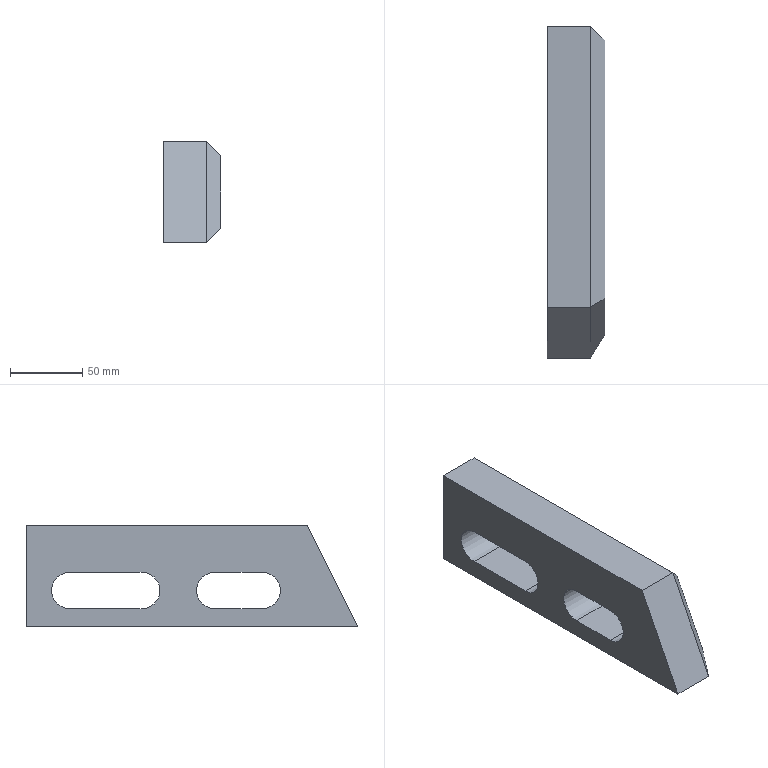Part | SolidWorks | features Chamfer 1, Extrusion 1 | 1 solid | 18 faces | box 40 x 229 x 70 mm | volume 442689 mm3 | plane 14 | cylinder 4 | commonest cylinder face diameters 25 x4
STEP:
#1=CARTESIAN_POINT('',(20.,184.,-10.));
#2=VERTEX_POINT('',#1);
#3=CARTESIAN_POINT('',(20.,6.18,-10.));
#4=VERTEX_POINT('',#3);
#5=CARTESIAN_POINT('',(20.,0.,-10.));
#6=DIRECTION('',(0.,-1.,0.));
#7=VECTOR('',#6,1000.);
#8=LINE('',#5,#7);
#9=EDGE_CURVE('',#2,#4,#8,.T.);
#10=ORIENTED_EDGE('',*,*,#9,.T.);
#11=CARTESIAN_POINT('',(20.,-18.82,-60.));
#12=VERTEX_POINT('',#11);
#13=CARTESIAN_POINT('',(20.,8.944,-4.472));
#14=DIRECTION('',(0.,-0.4472,-0.8944));
#15=VECTOR('',#14,1000.);
#16=LINE('',#13,#15);
#17=EDGE_CURVE('',#4,#12,#16,.T.);
#18=ORIENTED_EDGE('',*,*,#17,.T.);
#19=CARTESIAN_POINT('',(20.,184.,-60.));
#20=VERTEX_POINT('',#19);
#21=CARTESIAN_POINT('',(20.,0.,-60.));
#22=DIRECTION('',(0.,1.,0.));
#23=VECTOR('',#22,1000.);
#24=LINE('',#21,#23);
#25=EDGE_CURVE('',#12,#20,#24,.T.);
#26=ORIENTED_EDGE('',*,*,#25,.T.);
#27=CARTESIAN_POINT('',(20.,184.,0.));
#28=DIRECTION('',(0.,0.,1.));
#29=VECTOR('',#28,1000.);
#30=LINE('',#27,#29);
#31=EDGE_CURVE('',#20,#2,#30,.T.);
#32=ORIENTED_EDGE('',*,*,#31,.T.);
#33=EDGE_LOOP('',(#10,#18,#26,#32));
#34=FACE_OUTER_BOUND('',#33,.T.);
#35=CARTESIAN_POINT('',(20.,114.,-32.5));
#36=VERTEX_POINT('',#35);
#37=CARTESIAN_POINT('',(20.,114.,-57.5));
#38=VERTEX_POINT('',#37);
#39=CARTESIAN_POINT('',(20.,114.,-45.));
#40=DIRECTION('',(1.,0.,0.));
#41=DIRECTION('',(0.,0.,-1.));
#42=AXIS2_PLACEMENT_3D('',#39,#40,#41);
#43=CIRCLE('',#42,12.5);
#44=EDGE_CURVE('',#36,#38,#43,.T.);
#45=ORIENTED_EDGE('',*,*,#44,.F.);
#46=CARTESIAN_POINT('',(20.,164.,-32.5));
#47=VERTEX_POINT('',#46);
#48=CARTESIAN_POINT('',(20.,114.,-32.5));
#49=DIRECTION('',(0.,-1.,0.));
#50=VECTOR('',#49,1000.);
#51=LINE('',#48,#50);
#52=EDGE_CURVE('',#47,#36,#51,.T.);
#53=ORIENTED_EDGE('',*,*,#52,.F.);
#54=CARTESIAN_POINT('',(20.,164.,-57.5));
#55=VERTEX_POINT('',#54);
#56=CARTESIAN_POINT('',(20.,164.,-45.));
#57=DIRECTION('',(1.,0.,0.));
#58=DIRECTION('',(0.,0.,-1.));
#59=AXIS2_PLACEMENT_3D('',#56,#57,#58);
#60=CIRCLE('',#59,12.5);
#61=EDGE_CURVE('',#55,#47,#60,.T.);
#62=ORIENTED_EDGE('',*,*,#61,.F.);
#63=CARTESIAN_POINT('',(20.,114.,-57.5));
#64=DIRECTION('',(0.,1.,0.));
#65=VECTOR('',#64,1000.);
#66=LINE('',#63,#65);
#67=EDGE_CURVE('',#38,#55,#66,.T.);
#68=ORIENTED_EDGE('',*,*,#67,.F.);
#69=EDGE_LOOP('',(#45,#53,#62,#68));
#70=FACE_BOUND('',#69,.T.);
#71=CARTESIAN_POINT('',(20.,30.91,-32.5));
#72=VERTEX_POINT('',#71);
#73=CARTESIAN_POINT('',(20.,30.91,-57.5));
#74=VERTEX_POINT('',#73);
#75=CARTESIAN_POINT('',(20.,30.91,-45.));
#76=DIRECTION('',(1.,0.,0.));
#77=DIRECTION('',(0.,0.,-1.));
#78=AXIS2_PLACEMENT_3D('',#75,#76,#77);
#79=CIRCLE('',#78,12.5);
#80=EDGE_CURVE('',#72,#74,#79,.T.);
#81=ORIENTED_EDGE('',*,*,#80,.F.);
#82=CARTESIAN_POINT('',(20.,64.,-32.5));
#83=VERTEX_POINT('',#82);
#84=CARTESIAN_POINT('',(20.,30.91,-32.5));
#85=DIRECTION('',(0.,-1.,0.));
#86=VECTOR('',#85,1000.);
#87=LINE('',#84,#86);
#88=EDGE_CURVE('',#83,#72,#87,.T.);
#89=ORIENTED_EDGE('',*,*,#88,.F.);
#90=CARTESIAN_POINT('',(20.,64.,-57.5));
#91=VERTEX_POINT('',#90);
#92=CARTESIAN_POINT('',(20.,64.,-45.));
#93=DIRECTION('',(1.,0.,0.));
#94=DIRECTION('',(0.,0.,-1.));
#95=AXIS2_PLACEMENT_3D('',#92,#93,#94);
#96=CIRCLE('',#95,12.5);
#97=EDGE_CURVE('',#91,#83,#96,.T.);
#98=ORIENTED_EDGE('',*,*,#97,.F.);
#99=CARTESIAN_POINT('',(20.,30.91,-57.5));
#100=DIRECTION('',(0.,1.,0.));
#101=VECTOR('',#100,1000.);
#102=LINE('',#99,#101);
#103=EDGE_CURVE('',#74,#91,#102,.T.);
#104=ORIENTED_EDGE('',*,*,#103,.F.);
#105=EDGE_LOOP('',(#81,#89,#98,#104));
#106=FACE_BOUND('',#105,.T.);
#107=CARTESIAN_POINT('',(20.,0.,0.));
#108=DIRECTION('',(-1.,0.,0.));
#109=DIRECTION('',(0.,0.,1.));
#110=AXIS2_PLACEMENT_3D('',#107,#108,#109);
#111=PLANE('',#110);
#112=ADVANCED_FACE('',(#34,#70,#106),#111,.F.);
#113=CARTESIAN_POINT('',(-20.,194.,0.));
#114=VERTEX_POINT('',#113);
#115=CARTESIAN_POINT('',(-20.,0.,0.));
#116=VERTEX_POINT('',#115);
#117=CARTESIAN_POINT('',(-20.,194.,0.));
#118=DIRECTION('',(0.,-1.,0.));
#119=VECTOR('',#118,1000.);
#120=LINE('',#117,#119);
#121=EDGE_CURVE('',#114,#116,#120,.T.);
#122=ORIENTED_EDGE('',*,*,#121,.F.);
#123=CARTESIAN_POINT('',(-20.,194.,-70.));
#124=VERTEX_POINT('',#123);
#125=CARTESIAN_POINT('',(-20.,194.,-70.));
#126=DIRECTION('',(0.,0.,1.));
#127=VECTOR('',#126,1000.);
#128=LINE('',#125,#127);
#129=EDGE_CURVE('',#124,#114,#128,.T.);
#130=ORIENTED_EDGE('',*,*,#129,.F.);
#131=CARTESIAN_POINT('',(-20.,-35.,-70.));
#132=VERTEX_POINT('',#131);
#133=CARTESIAN_POINT('',(-20.,-35.,-70.));
#134=DIRECTION('',(0.,1.,0.));
#135=VECTOR('',#134,1000.);
#136=LINE('',#133,#135);
#137=EDGE_CURVE('',#132,#124,#136,.T.);
#138=ORIENTED_EDGE('',*,*,#137,.F.);
#139=CARTESIAN_POINT('',(-20.,0.,0.));
#140=DIRECTION('',(0.,-0.4472,-0.8944));
#141=VECTOR('',#140,1000.);
#142=LINE('',#139,#141);
#143=EDGE_CURVE('',#116,#132,#142,.T.);
#144=ORIENTED_EDGE('',*,*,#143,.F.);
#145=EDGE_LOOP('',(#122,#130,#138,#144));
#146=FACE_OUTER_BOUND('',#145,.T.);
#147=CARTESIAN_POINT('',(-20.,164.,-32.5));
#148=VERTEX_POINT('',#147);
#149=CARTESIAN_POINT('',(-20.,114.,-32.5));
#150=VERTEX_POINT('',#149);
#151=CARTESIAN_POINT('',(-20.,114.,-32.5));
#152=DIRECTION('',(0.,-1.,0.));
#153=VECTOR('',#152,1000.);
#154=LINE('',#151,#153);
#155=EDGE_CURVE('',#148,#150,#154,.T.);
#156=ORIENTED_EDGE('',*,*,#155,.T.);
#157=CARTESIAN_POINT('',(-20.,114.,-57.5));
#158=VERTEX_POINT('',#157);
#159=CARTESIAN_POINT('',(-20.,114.,-45.));
#160=DIRECTION('',(1.,0.,0.));
#161=DIRECTION('',(0.,0.,-1.));
#162=AXIS2_PLACEMENT_3D('',#159,#160,#161);
#163=CIRCLE('',#162,12.5);
#164=EDGE_CURVE('',#150,#158,#163,.T.);
#165=ORIENTED_EDGE('',*,*,#164,.T.);
#166=CARTESIAN_POINT('',(-20.,164.,-57.5));
#167=VERTEX_POINT('',#166);
#168=CARTESIAN_POINT('',(-20.,114.,-57.5));
#169=DIRECTION('',(0.,1.,0.));
#170=VECTOR('',#169,1000.);
#171=LINE('',#168,#170);
#172=EDGE_CURVE('',#158,#167,#171,.T.);
#173=ORIENTED_EDGE('',*,*,#172,.T.);
#174=CARTESIAN_POINT('',(-20.,164.,-45.));
#175=DIRECTION('',(1.,0.,0.));
#176=DIRECTION('',(0.,0.,-1.));
#177=AXIS2_PLACEMENT_3D('',#174,#175,#176);
#178=CIRCLE('',#177,12.5);
#179=EDGE_CURVE('',#167,#148,#178,.T.);
#180=ORIENTED_EDGE('',*,*,#179,.T.);
#181=EDGE_LOOP('',(#156,#165,#173,#180));
#182=FACE_BOUND('',#181,.T.);
#183=CARTESIAN_POINT('',(-20.,64.,-32.5));
#184=VERTEX_POINT('',#183);
#185=CARTESIAN_POINT('',(-20.,30.91,-32.5));
#186=VERTEX_POINT('',#185);
#187=CARTESIAN_POINT('',(-20.,30.91,-32.5));
#188=DIRECTION('',(0.,-1.,0.));
#189=VECTOR('',#188,1000.);
#190=LINE('',#187,#189);
#191=EDGE_CURVE('',#184,#186,#190,.T.);
#192=ORIENTED_EDGE('',*,*,#191,.T.);
#193=CARTESIAN_POINT('',(-20.,30.91,-57.5));
#194=VERTEX_POINT('',#193);
#195=CARTESIAN_POINT('',(-20.,30.91,-45.));
#196=DIRECTION('',(1.,0.,0.));
#197=DIRECTION('',(0.,0.,-1.));
#198=AXIS2_PLACEMENT_3D('',#195,#196,#197);
#199=CIRCLE('',#198,12.5);
#200=EDGE_CURVE('',#186,#194,#199,.T.);
#201=ORIENTED_EDGE('',*,*,#200,.T.);
#202=CARTESIAN_POINT('',(-20.,64.,-57.5));
#203=VERTEX_POINT('',#202);
#204=CARTESIAN_POINT('',(-20.,30.91,-57.5));
#205=DIRECTION('',(0.,1.,0.));
#206=VECTOR('',#205,1000.);
#207=LINE('',#204,#206);
#208=EDGE_CURVE('',#194,#203,#207,.T.);
#209=ORIENTED_EDGE('',*,*,#208,.T.);
#210=CARTESIAN_POINT('',(-20.,64.,-45.));
#211=DIRECTION('',(1.,0.,0.));
#212=DIRECTION('',(0.,0.,-1.));
#213=AXIS2_PLACEMENT_3D('',#210,#211,#212);
#214=CIRCLE('',#213,12.5);
#215=EDGE_CURVE('',#203,#184,#214,.T.);
#216=ORIENTED_EDGE('',*,*,#215,.T.);
#217=EDGE_LOOP('',(#192,#201,#209,#216));
#218=FACE_BOUND('',#217,.T.);
#219=CARTESIAN_POINT('',(-20.,0.,0.));
#220=DIRECTION('',(-1.,0.,0.));
#221=DIRECTION('',(0.,0.,1.));
#222=AXIS2_PLACEMENT_3D('',#219,#220,#221);
#223=PLANE('',#222);
#224=ADVANCED_FACE('',(#146,#182,#218),#223,.T.);
#225=CARTESIAN_POINT('',(10.,0.,0.));
#226=VERTEX_POINT('',#225);
#227=CARTESIAN_POINT('',(20.,0.,0.));
#228=DIRECTION('',(-1.,0.,0.));
#229=VECTOR('',#228,1000.);
#230=LINE('',#227,#229);
#231=EDGE_CURVE('',#226,#116,#230,.T.);
#232=ORIENTED_EDGE('',*,*,#231,.F.);
#233=CARTESIAN_POINT('',(10.,194.,0.));
#234=VERTEX_POINT('',#233);
#235=CARTESIAN_POINT('',(10.,194.,0.));
#236=DIRECTION('',(0.,1.,0.));
#237=VECTOR('',#236,1000.);
#238=LINE('',#235,#237);
#239=EDGE_CURVE('',#226,#234,#238,.T.);
#240=ORIENTED_EDGE('',*,*,#239,.T.);
#241=CARTESIAN_POINT('',(20.,194.,0.));
#242=DIRECTION('',(-1.,0.,0.));
#243=VECTOR('',#242,1000.);
#244=LINE('',#241,#243);
#245=EDGE_CURVE('',#234,#114,#244,.T.);
#246=ORIENTED_EDGE('',*,*,#245,.T.);
#247=ORIENTED_EDGE('',*,*,#121,.T.);
#248=EDGE_LOOP('',(#232,#240,#246,#247));
#249=FACE_OUTER_BOUND('',#248,.T.);
#250=CARTESIAN_POINT('',(20.,194.,0.));
#251=DIRECTION('',(0.,0.,-1.));
#252=DIRECTION('',(-1.,0.,0.));
#253=AXIS2_PLACEMENT_3D('',#250,#251,#252);
#254=PLANE('',#253);
#255=ADVANCED_FACE('',(#249),#254,.F.);
#256=CARTESIAN_POINT('',(10.,-35.,-70.));
#257=VERTEX_POINT('',#256);
#258=CARTESIAN_POINT('',(20.,-35.,-70.));
#259=DIRECTION('',(-1.,0.,0.));
#260=VECTOR('',#259,1000.);
#261=LINE('',#258,#260);
#262=EDGE_CURVE('',#257,#132,#261,.T.);
#263=ORIENTED_EDGE('',*,*,#262,.F.);
#264=CARTESIAN_POINT('',(10.,0.,0.));
#265=DIRECTION('',(0.,0.4472,0.8944));
#266=VECTOR('',#265,1000.);
#267=LINE('',#264,#266);
#268=EDGE_CURVE('',#257,#226,#267,.T.);
#269=ORIENTED_EDGE('',*,*,#268,.T.);
#270=ORIENTED_EDGE('',*,*,#231,.T.);
#271=ORIENTED_EDGE('',*,*,#143,.T.);
#272=EDGE_LOOP('',(#263,#269,#270,#271));
#273=FACE_OUTER_BOUND('',#272,.T.);
#274=CARTESIAN_POINT('',(20.,0.,0.));
#275=DIRECTION('',(0.,0.8944,-0.4472));
#276=DIRECTION('',(0.,0.4472,0.8944));
#277=AXIS2_PLACEMENT_3D('',#274,#275,#276);
#278=PLANE('',#277);
#279=ADVANCED_FACE('',(#273),#278,.F.);
#280=CARTESIAN_POINT('',(10.,194.,-70.));
#281=VERTEX_POINT('',#280);
#282=CARTESIAN_POINT('',(20.,194.,-70.));
#283=DIRECTION('',(-1.,0.,0.));
#284=VECTOR('',#283,1000.);
#285=LINE('',#282,#284);
#286=EDGE_CURVE('',#281,#124,#285,.T.);
#287=ORIENTED_EDGE('',*,*,#286,.F.);
#288=CARTESIAN_POINT('',(10.,-35.,-70.));
#289=DIRECTION('',(0.,-1.,0.));
#290=VECTOR('',#289,1000.);
#291=LINE('',#288,#290);
#292=EDGE_CURVE('',#281,#257,#291,.T.);
#293=ORIENTED_EDGE('',*,*,#292,.T.);
#294=ORIENTED_EDGE('',*,*,#262,.T.);
#295=ORIENTED_EDGE('',*,*,#137,.T.);
#296=EDGE_LOOP('',(#287,#293,#294,#295));
#297=FACE_OUTER_BOUND('',#296,.T.);
#298=CARTESIAN_POINT('',(20.,-35.,-70.));
#299=DIRECTION('',(0.,0.,1.));
#300=DIRECTION('',(0.,-1.,0.));
#301=AXIS2_PLACEMENT_3D('',#298,#299,#300);
#302=PLANE('',#301);
#303=ADVANCED_FACE('',(#297),#302,.F.);
#304=ORIENTED_EDGE('',*,*,#245,.F.);
#305=CARTESIAN_POINT('',(10.,194.,-70.));
#306=DIRECTION('',(0.,0.,-1.));
#307=VECTOR('',#306,1000.);
#308=LINE('',#305,#307);
#309=EDGE_CURVE('',#234,#281,#308,.T.);
#310=ORIENTED_EDGE('',*,*,#309,.T.);
#311=ORIENTED_EDGE('',*,*,#286,.T.);
#312=ORIENTED_EDGE('',*,*,#129,.T.);
#313=EDGE_LOOP('',(#304,#310,#311,#312));
#314=FACE_OUTER_BOUND('',#313,.T.);
#315=CARTESIAN_POINT('',(20.,194.,-70.));
#316=DIRECTION('',(0.,-1.,0.));
#317=DIRECTION('',(0.,0.,-1.));
#318=AXIS2_PLACEMENT_3D('',#315,#316,#317);
#319=PLANE('',#318);
#320=ADVANCED_FACE('',(#314),#319,.F.);
#321=ORIENTED_EDGE('',*,*,#164,.F.);
#322=CARTESIAN_POINT('',(20.,114.,-32.5));
#323=DIRECTION('',(-1.,0.,0.));
#324=VECTOR('',#323,1000.);
#325=LINE('',#322,#324);
#326=EDGE_CURVE('',#36,#150,#325,.T.);
#327=ORIENTED_EDGE('',*,*,#326,.F.);
#328=ORIENTED_EDGE('',*,*,#44,.T.);
#329=CARTESIAN_POINT('',(20.,114.,-57.5));
#330=DIRECTION('',(-1.,0.,0.));
#331=VECTOR('',#330,1000.);
#332=LINE('',#329,#331);
#333=EDGE_CURVE('',#38,#158,#332,.T.);
#334=ORIENTED_EDGE('',*,*,#333,.T.);
#335=EDGE_LOOP('',(#321,#327,#328,#334));
#336=FACE_OUTER_BOUND('',#335,.T.);
#337=CARTESIAN_POINT('',(20.,114.,-45.));
#338=DIRECTION('',(-1.,0.,0.));
#339=DIRECTION('',(0.,0.,1.));
#340=AXIS2_PLACEMENT_3D('',#337,#338,#339);
#341=CYLINDRICAL_SURFACE('',#340,12.5);
#342=ADVANCED_FACE('',(#336),#341,.F.);
#343=ORIENTED_EDGE('',*,*,#172,.F.);
#344=ORIENTED_EDGE('',*,*,#333,.F.);
#345=ORIENTED_EDGE('',*,*,#67,.T.);
#346=CARTESIAN_POINT('',(20.,164.,-57.5));
#347=DIRECTION('',(-1.,0.,0.));
#348=VECTOR('',#347,1000.);
#349=LINE('',#346,#348);
#350=EDGE_CURVE('',#55,#167,#349,.T.);
#351=ORIENTED_EDGE('',*,*,#350,.T.);
#352=EDGE_LOOP('',(#343,#344,#345,#351));
#353=FACE_OUTER_BOUND('',#352,.T.);
#354=CARTESIAN_POINT('',(20.,114.,-57.5));
#355=DIRECTION('',(0.,0.,1.));
#356=DIRECTION('',(1.,0.,0.));
#357=AXIS2_PLACEMENT_3D('',#354,#355,#356);
#358=PLANE('',#357);
#359=ADVANCED_FACE('',(#353),#358,.T.);
#360=ORIENTED_EDGE('',*,*,#179,.F.);
#361=ORIENTED_EDGE('',*,*,#350,.F.);
#362=ORIENTED_EDGE('',*,*,#61,.T.);
#363=CARTESIAN_POINT('',(20.,164.,-32.5));
#364=DIRECTION('',(-1.,0.,0.));
#365=VECTOR('',#364,1000.);
#366=LINE('',#363,#365);
#367=EDGE_CURVE('',#47,#148,#366,.T.);
#368=ORIENTED_EDGE('',*,*,#367,.T.);
#369=EDGE_LOOP('',(#360,#361,#362,#368));
#370=FACE_OUTER_BOUND('',#369,.T.);
#371=CARTESIAN_POINT('',(20.,164.,-45.));
#372=DIRECTION('',(-1.,0.,0.));
#373=DIRECTION('',(0.,0.,1.));
#374=AXIS2_PLACEMENT_3D('',#371,#372,#373);
#375=CYLINDRICAL_SURFACE('',#374,12.5);
#376=ADVANCED_FACE('',(#370),#375,.F.);
#377=ORIENTED_EDGE('',*,*,#155,.F.);
#378=ORIENTED_EDGE('',*,*,#367,.F.);
#379=ORIENTED_EDGE('',*,*,#52,.T.);
#380=ORIENTED_EDGE('',*,*,#326,.T.);
#381=EDGE_LOOP('',(#377,#378,#379,#380));
#382=FACE_OUTER_BOUND('',#381,.T.);
#383=CARTESIAN_POINT('',(20.,114.,-32.5));
#384=DIRECTION('',(0.,0.,-1.));
#385=DIRECTION('',(-1.,0.,0.));
#386=AXIS2_PLACEMENT_3D('',#383,#384,#385);
#387=PLANE('',#386);
#388=ADVANCED_FACE('',(#382),#387,.T.);
#389=ORIENTED_EDGE('',*,*,#200,.F.);
#390=CARTESIAN_POINT('',(20.,30.91,-32.5));
#391=DIRECTION('',(-1.,0.,0.));
#392=VECTOR('',#391,1000.);
#393=LINE('',#390,#392);
#394=EDGE_CURVE('',#72,#186,#393,.T.);
#395=ORIENTED_EDGE('',*,*,#394,.F.);
#396=ORIENTED_EDGE('',*,*,#80,.T.);
#397=CARTESIAN_POINT('',(20.,30.91,-57.5));
#398=DIRECTION('',(-1.,0.,0.));
#399=VECTOR('',#398,1000.);
#400=LINE('',#397,#399);
#401=EDGE_CURVE('',#74,#194,#400,.T.);
#402=ORIENTED_EDGE('',*,*,#401,.T.);
#403=EDGE_LOOP('',(#389,#395,#396,#402));
#404=FACE_OUTER_BOUND('',#403,.T.);
#405=CARTESIAN_POINT('',(20.,30.91,-45.));
#406=DIRECTION('',(-1.,0.,0.));
#407=DIRECTION('',(0.,0.,1.));
#408=AXIS2_PLACEMENT_3D('',#405,#406,#407);
#409=CYLINDRICAL_SURFACE('',#408,12.5);
#410=ADVANCED_FACE('',(#404),#409,.F.);
#411=ORIENTED_EDGE('',*,*,#208,.F.);
#412=ORIENTED_EDGE('',*,*,#401,.F.);
#413=ORIENTED_EDGE('',*,*,#103,.T.);
#414=CARTESIAN_POINT('',(20.,64.,-57.5));
#415=DIRECTION('',(-1.,0.,0.));
#416=VECTOR('',#415,1000.);
#417=LINE('',#414,#416);
#418=EDGE_CURVE('',#91,#203,#417,.T.);
#419=ORIENTED_EDGE('',*,*,#418,.T.);
#420=EDGE_LOOP('',(#411,#412,#413,#419));
#421=FACE_OUTER_BOUND('',#420,.T.);
#422=CARTESIAN_POINT('',(20.,30.91,-57.5));
#423=DIRECTION('',(0.,0.,1.));
#424=DIRECTION('',(1.,0.,0.));
#425=AXIS2_PLACEMENT_3D('',#422,#423,#424);
#426=PLANE('',#425);
#427=ADVANCED_FACE('',(#421),#426,.T.);
#428=ORIENTED_EDGE('',*,*,#215,.F.);
#429=ORIENTED_EDGE('',*,*,#418,.F.);
#430=ORIENTED_EDGE('',*,*,#97,.T.);
#431=CARTESIAN_POINT('',(20.,64.,-32.5));
#432=DIRECTION('',(-1.,0.,0.));
#433=VECTOR('',#432,1000.);
#434=LINE('',#431,#433);
#435=EDGE_CURVE('',#83,#184,#434,.T.);
#436=ORIENTED_EDGE('',*,*,#435,.T.);
#437=EDGE_LOOP('',(#428,#429,#430,#436));
#438=FACE_OUTER_BOUND('',#437,.T.);
#439=CARTESIAN_POINT('',(20.,64.,-45.));
#440=DIRECTION('',(-1.,0.,0.));
#441=DIRECTION('',(0.,0.,1.));
#442=AXIS2_PLACEMENT_3D('',#439,#440,#441);
#443=CYLINDRICAL_SURFACE('',#442,12.5);
#444=ADVANCED_FACE('',(#438),#443,.F.);
#445=ORIENTED_EDGE('',*,*,#191,.F.);
#446=ORIENTED_EDGE('',*,*,#435,.F.);
#447=ORIENTED_EDGE('',*,*,#88,.T.);
#448=ORIENTED_EDGE('',*,*,#394,.T.);
#449=EDGE_LOOP('',(#445,#446,#447,#448));
#450=FACE_OUTER_BOUND('',#449,.T.);
#451=CARTESIAN_POINT('',(20.,30.91,-32.5));
#452=DIRECTION('',(0.,0.,-1.));
#453=DIRECTION('',(-1.,0.,0.));
#454=AXIS2_PLACEMENT_3D('',#451,#452,#453);
#455=PLANE('',#454);
#456=ADVANCED_FACE('',(#450),#455,.T.);
#457=CARTESIAN_POINT('',(40.,164.,-40.));
#458=DIRECTION('',(0.5774,-0.5774,0.5774));
#459=VECTOR('',#458,1000.);
#460=LINE('',#457,#459);
#461=EDGE_CURVE('',#281,#20,#460,.T.);
#462=ORIENTED_EDGE('',*,*,#461,.F.);
#463=ORIENTED_EDGE('',*,*,#309,.F.);
#464=CARTESIAN_POINT('',(16.667,187.333,-6.667));
#465=DIRECTION('',(-0.5774,0.5774,0.5774));
#466=VECTOR('',#465,1000.);
#467=LINE('',#464,#466);
#468=EDGE_CURVE('',#2,#234,#467,.T.);
#469=ORIENTED_EDGE('',*,*,#468,.F.);
#470=ORIENTED_EDGE('',*,*,#31,.F.);
#471=EDGE_LOOP('',(#462,#463,#469,#470));
#472=FACE_OUTER_BOUND('',#471,.T.);
#473=CARTESIAN_POINT('',(20.,184.,0.));
#474=DIRECTION('',(-0.7071,-0.7071,0.));
#475=DIRECTION('',(0.,0.,1.));
#476=AXIS2_PLACEMENT_3D('',#473,#474,#475);
#477=PLANE('',#476);
#478=ADVANCED_FACE('',(#472),#477,.F.);
#479=ORIENTED_EDGE('',*,*,#468,.T.);
#480=ORIENTED_EDGE('',*,*,#239,.F.);
#481=CARTESIAN_POINT('',(18.396,5.189,-8.396));
#482=DIRECTION('',(-0.6479,-0.4004,0.6479));
#483=VECTOR('',#482,1000.);
#484=LINE('',#481,#483);
#485=EDGE_CURVE('',#4,#226,#484,.T.);
#486=ORIENTED_EDGE('',*,*,#485,.F.);
#487=ORIENTED_EDGE('',*,*,#9,.F.);
#488=EDGE_LOOP('',(#479,#480,#486,#487));
#489=FACE_OUTER_BOUND('',#488,.T.);
#490=CARTESIAN_POINT('',(20.,0.,-10.));
#491=DIRECTION('',(-0.7071,0.,-0.7071));
#492=DIRECTION('',(0.,-1.,0.));
#493=AXIS2_PLACEMENT_3D('',#490,#491,#492);
#494=PLANE('',#493);
#495=ADVANCED_FACE('',(#489),#494,.F.);
#496=ORIENTED_EDGE('',*,*,#461,.T.);
#497=ORIENTED_EDGE('',*,*,#25,.F.);
#498=CARTESIAN_POINT('',(26.594,-8.151,-53.406));
#499=DIRECTION('',(0.4653,0.7529,0.4653));
#500=VECTOR('',#499,1000.);
#501=LINE('',#498,#500);
#502=EDGE_CURVE('',#257,#12,#501,.T.);
#503=ORIENTED_EDGE('',*,*,#502,.F.);
#504=ORIENTED_EDGE('',*,*,#292,.F.);
#505=EDGE_LOOP('',(#496,#497,#503,#504));
#506=FACE_OUTER_BOUND('',#505,.T.);
#507=CARTESIAN_POINT('',(20.,0.,-60.));
#508=DIRECTION('',(-0.7071,0.,0.7071));
#509=DIRECTION('',(0.,1.,0.));
#510=AXIS2_PLACEMENT_3D('',#507,#508,#509);
#511=PLANE('',#510);
#512=ADVANCED_FACE('',(#506),#511,.F.);
#513=ORIENTED_EDGE('',*,*,#485,.T.);
#514=ORIENTED_EDGE('',*,*,#268,.F.);
#515=ORIENTED_EDGE('',*,*,#502,.T.);
#516=ORIENTED_EDGE('',*,*,#17,.F.);
#517=EDGE_LOOP('',(#513,#514,#515,#516));
#518=FACE_OUTER_BOUND('',#517,.T.);
#519=CARTESIAN_POINT('',(20.,8.944,-4.472));
#520=DIRECTION('',(-0.7071,0.6325,-0.3162));
#521=DIRECTION('',(0.,-0.4472,-0.8944));
#522=AXIS2_PLACEMENT_3D('',#519,#520,#521);
#523=PLANE('',#522);
#524=ADVANCED_FACE('',(#518),#523,.F.);
#525=CLOSED_SHELL('',(#112,#224,#255,#279,#303,#320,#342,#359,#376,#388,#410,#427,#444,#456,#478,#495,#512,#524));
#526=MANIFOLD_SOLID_BREP('',#525);
#527=CARTESIAN_POINT('',(0.,0.,0.));
#528=DIRECTION('',(0.,0.,1.));
#529=DIRECTION('',(1.,0.,0.));
#530=AXIS2_PLACEMENT_3D('',#527,#528,#529);
#531=(LENGTH_UNIT()NAMED_UNIT(*)SI_UNIT(.MILLI.,.METRE.));
#532=UNCERTAINTY_MEASURE_WITH_UNIT(LENGTH_MEASURE(0.00001),#531,'','');
#533=(NAMED_UNIT(*)PLANE_ANGLE_UNIT()SI_UNIT($,.RADIAN.));
#534=(NAMED_UNIT(*)SI_UNIT($,.STERADIAN.)SOLID_ANGLE_UNIT());
#535=(GEOMETRIC_REPRESENTATION_CONTEXT(3)GLOBAL_UNCERTAINTY_ASSIGNED_CONTEXT((#532))GLOBAL_UNIT_ASSIGNED_CONTEXT((#531,#533,#534))REPRESENTATION_CONTEXT('',''));
#536=ADVANCED_BREP_SHAPE_REPRESENTATION('',(#526,#530),#535);